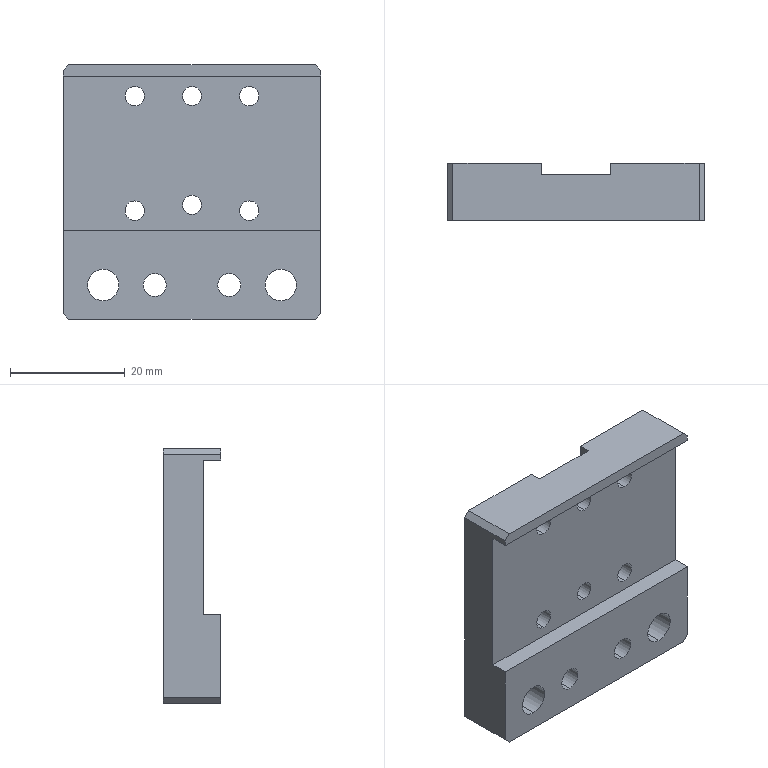Part | STEP file | PN_0007 | 1 solid | 58 faces | box 45 x 10 x 44.5 mm | volume 13324 mm3 | cylinder 32 | plane 26 | commonest cylinder face diameters 3.4 x8 6.5 x8 3.3 x4 4 x4 5.5 x4 10 x4